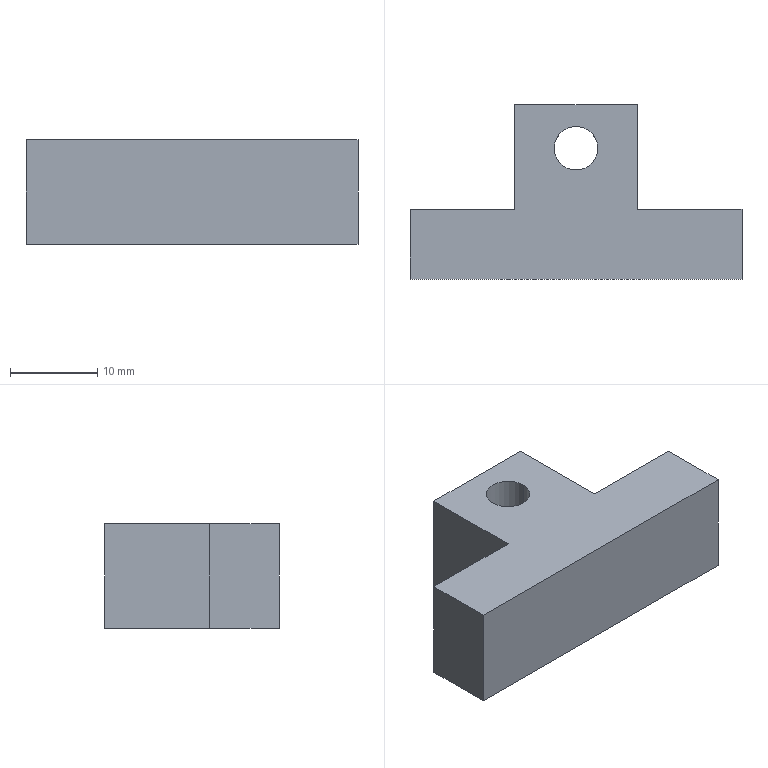Part | SolidWorks | features 3DProfileFeature 1, Extrusion 1, HoleWzd 1 | 1 solid | 12 faces | box 38 x 20 x 12 mm | volume 5428 mm3 | plane 10 | cylinder 2 | commonest cylinder face diameters 5 x2
STEP:
#1=CARTESIAN_POINT('',(-2.5,-5.,-6.));
#2=VERTEX_POINT('',#1);
#3=CARTESIAN_POINT('',(2.5,-5.,-6.));
#4=VERTEX_POINT('',#3);
#5=CARTESIAN_POINT('',(0.,-5.,-6.));
#6=DIRECTION('',(0.,0.,1.));
#7=DIRECTION('',(1.,0.,0.));
#8=AXIS2_PLACEMENT_3D('',#5,#6,#7);
#9=CIRCLE('',#8,2.5);
#10=EDGE_CURVE('',#2,#4,#9,.T.);
#11=ORIENTED_EDGE('',*,*,#10,.F.);
#12=CARTESIAN_POINT('',(-2.5,-5.,6.));
#13=VERTEX_POINT('',#12);
#14=CARTESIAN_POINT('',(-2.5,-5.,6.));
#15=DIRECTION('',(0.,0.,1.));
#16=VECTOR('',#15,1000.);
#17=LINE('',#14,#16);
#18=EDGE_CURVE('',#2,#13,#17,.T.);
#19=ORIENTED_EDGE('',*,*,#18,.T.);
#20=CARTESIAN_POINT('',(2.5,-5.,6.));
#21=VERTEX_POINT('',#20);
#22=CARTESIAN_POINT('',(0.,-5.,6.));
#23=DIRECTION('',(0.,0.,1.));
#24=DIRECTION('',(1.,0.,0.));
#25=AXIS2_PLACEMENT_3D('',#22,#23,#24);
#26=CIRCLE('',#25,2.5);
#27=EDGE_CURVE('',#13,#21,#26,.T.);
#28=ORIENTED_EDGE('',*,*,#27,.T.);
#29=CARTESIAN_POINT('',(2.5,-5.,6.));
#30=DIRECTION('',(0.,0.,1.));
#31=VECTOR('',#30,1000.);
#32=LINE('',#29,#31);
#33=EDGE_CURVE('',#4,#21,#32,.T.);
#34=ORIENTED_EDGE('',*,*,#33,.F.);
#35=EDGE_LOOP('',(#11,#19,#28,#34));
#36=FACE_OUTER_BOUND('',#35,.T.);
#37=CARTESIAN_POINT('',(0.,-5.,6.));
#38=DIRECTION('',(0.,0.,1.));
#39=DIRECTION('',(1.,0.,0.));
#40=AXIS2_PLACEMENT_3D('',#37,#38,#39);
#41=CYLINDRICAL_SURFACE('',#40,2.5);
#42=ADVANCED_FACE('',(#36),#41,.F.);
#43=CARTESIAN_POINT('',(7.,0.,-6.));
#44=VERTEX_POINT('',#43);
#45=CARTESIAN_POINT('',(-7.,0.,-6.));
#46=VERTEX_POINT('',#45);
#47=CARTESIAN_POINT('',(0.,0.,-6.));
#48=DIRECTION('',(-1.,0.,0.));
#49=VECTOR('',#48,1000.);
#50=LINE('',#47,#49);
#51=EDGE_CURVE('',#44,#46,#50,.T.);
#52=ORIENTED_EDGE('',*,*,#51,.T.);
#53=CARTESIAN_POINT('',(-7.,0.,6.));
#54=VERTEX_POINT('',#53);
#55=CARTESIAN_POINT('',(-7.,0.,6.));
#56=DIRECTION('',(0.,0.,-1.));
#57=VECTOR('',#56,1000.);
#58=LINE('',#55,#57);
#59=EDGE_CURVE('',#54,#46,#58,.T.);
#60=ORIENTED_EDGE('',*,*,#59,.F.);
#61=CARTESIAN_POINT('',(7.,0.,6.));
#62=VERTEX_POINT('',#61);
#63=CARTESIAN_POINT('',(7.,0.,6.));
#64=DIRECTION('',(-1.,0.,0.));
#65=VECTOR('',#64,1000.);
#66=LINE('',#63,#65);
#67=EDGE_CURVE('',#62,#54,#66,.T.);
#68=ORIENTED_EDGE('',*,*,#67,.F.);
#69=CARTESIAN_POINT('',(7.,0.,6.));
#70=DIRECTION('',(0.,0.,-1.));
#71=VECTOR('',#70,1000.);
#72=LINE('',#69,#71);
#73=EDGE_CURVE('',#62,#44,#72,.T.);
#74=ORIENTED_EDGE('',*,*,#73,.T.);
#75=EDGE_LOOP('',(#52,#60,#68,#74));
#76=FACE_OUTER_BOUND('',#75,.T.);
#77=CARTESIAN_POINT('',(0.,0.,6.));
#78=DIRECTION('',(0.,-1.,0.));
#79=DIRECTION('',(0.,0.,-1.));
#80=AXIS2_PLACEMENT_3D('',#77,#78,#79);
#81=PLANE('',#80);
#82=ADVANCED_FACE('',(#76),#81,.F.);
#83=CARTESIAN_POINT('',(-7.,-12.,-6.));
#84=VERTEX_POINT('',#83);
#85=CARTESIAN_POINT('',(-7.,0.,-6.));
#86=DIRECTION('',(0.,-1.,0.));
#87=VECTOR('',#86,1000.);
#88=LINE('',#85,#87);
#89=EDGE_CURVE('',#46,#84,#88,.T.);
#90=ORIENTED_EDGE('',*,*,#89,.T.);
#91=CARTESIAN_POINT('',(-7.,-12.,6.));
#92=VERTEX_POINT('',#91);
#93=CARTESIAN_POINT('',(-7.,-12.,6.));
#94=DIRECTION('',(0.,0.,-1.));
#95=VECTOR('',#94,1000.);
#96=LINE('',#93,#95);
#97=EDGE_CURVE('',#92,#84,#96,.T.);
#98=ORIENTED_EDGE('',*,*,#97,.F.);
#99=CARTESIAN_POINT('',(-7.,0.,6.));
#100=DIRECTION('',(0.,-1.,0.));
#101=VECTOR('',#100,1000.);
#102=LINE('',#99,#101);
#103=EDGE_CURVE('',#54,#92,#102,.T.);
#104=ORIENTED_EDGE('',*,*,#103,.F.);
#105=ORIENTED_EDGE('',*,*,#59,.T.);
#106=EDGE_LOOP('',(#90,#98,#104,#105));
#107=FACE_OUTER_BOUND('',#106,.T.);
#108=CARTESIAN_POINT('',(-7.,0.,6.));
#109=DIRECTION('',(1.,0.,0.));
#110=DIRECTION('',(0.,1.,0.));
#111=AXIS2_PLACEMENT_3D('',#108,#109,#110);
#112=PLANE('',#111);
#113=ADVANCED_FACE('',(#107),#112,.F.);
#114=CARTESIAN_POINT('',(-19.,-12.,-6.));
#115=VERTEX_POINT('',#114);
#116=CARTESIAN_POINT('',(-7.,-12.,-6.));
#117=DIRECTION('',(-1.,0.,0.));
#118=VECTOR('',#117,1000.);
#119=LINE('',#116,#118);
#120=EDGE_CURVE('',#84,#115,#119,.T.);
#121=ORIENTED_EDGE('',*,*,#120,.T.);
#122=CARTESIAN_POINT('',(-19.,-12.,6.));
#123=VERTEX_POINT('',#122);
#124=CARTESIAN_POINT('',(-19.,-12.,6.));
#125=DIRECTION('',(0.,0.,-1.));
#126=VECTOR('',#125,1000.);
#127=LINE('',#124,#126);
#128=EDGE_CURVE('',#123,#115,#127,.T.);
#129=ORIENTED_EDGE('',*,*,#128,.F.);
#130=CARTESIAN_POINT('',(-7.,-12.,6.));
#131=DIRECTION('',(-1.,0.,0.));
#132=VECTOR('',#131,1000.);
#133=LINE('',#130,#132);
#134=EDGE_CURVE('',#92,#123,#133,.T.);
#135=ORIENTED_EDGE('',*,*,#134,.F.);
#136=ORIENTED_EDGE('',*,*,#97,.T.);
#137=EDGE_LOOP('',(#121,#129,#135,#136));
#138=FACE_OUTER_BOUND('',#137,.T.);
#139=CARTESIAN_POINT('',(-7.,-12.,6.));
#140=DIRECTION('',(0.,-1.,0.));
#141=DIRECTION('',(1.,0.,0.));
#142=AXIS2_PLACEMENT_3D('',#139,#140,#141);
#143=PLANE('',#142);
#144=ADVANCED_FACE('',(#138),#143,.F.);
#145=CARTESIAN_POINT('',(-19.,-20.,-6.));
#146=VERTEX_POINT('',#145);
#147=CARTESIAN_POINT('',(-19.,-12.,-6.));
#148=DIRECTION('',(0.,-1.,0.));
#149=VECTOR('',#148,1000.);
#150=LINE('',#147,#149);
#151=EDGE_CURVE('',#115,#146,#150,.T.);
#152=ORIENTED_EDGE('',*,*,#151,.T.);
#153=CARTESIAN_POINT('',(-19.,-20.,6.));
#154=VERTEX_POINT('',#153);
#155=CARTESIAN_POINT('',(-19.,-20.,6.));
#156=DIRECTION('',(0.,0.,-1.));
#157=VECTOR('',#156,1000.);
#158=LINE('',#155,#157);
#159=EDGE_CURVE('',#154,#146,#158,.T.);
#160=ORIENTED_EDGE('',*,*,#159,.F.);
#161=CARTESIAN_POINT('',(-19.,-12.,6.));
#162=DIRECTION('',(0.,-1.,0.));
#163=VECTOR('',#162,1000.);
#164=LINE('',#161,#163);
#165=EDGE_CURVE('',#123,#154,#164,.T.);
#166=ORIENTED_EDGE('',*,*,#165,.F.);
#167=ORIENTED_EDGE('',*,*,#128,.T.);
#168=EDGE_LOOP('',(#152,#160,#166,#167));
#169=FACE_OUTER_BOUND('',#168,.T.);
#170=CARTESIAN_POINT('',(-19.,-12.,6.));
#171=DIRECTION('',(1.,0.,0.));
#172=DIRECTION('',(0.,0.,-1.));
#173=AXIS2_PLACEMENT_3D('',#170,#171,#172);
#174=PLANE('',#173);
#175=ADVANCED_FACE('',(#169),#174,.F.);
#176=CARTESIAN_POINT('',(19.,-20.,-6.));
#177=VERTEX_POINT('',#176);
#178=CARTESIAN_POINT('',(-19.,-20.,-6.));
#179=DIRECTION('',(1.,0.,0.));
#180=VECTOR('',#179,1000.);
#181=LINE('',#178,#180);
#182=EDGE_CURVE('',#146,#177,#181,.T.);
#183=ORIENTED_EDGE('',*,*,#182,.T.);
#184=CARTESIAN_POINT('',(19.,-20.,6.));
#185=VERTEX_POINT('',#184);
#186=CARTESIAN_POINT('',(19.,-20.,6.));
#187=DIRECTION('',(0.,0.,-1.));
#188=VECTOR('',#187,1000.);
#189=LINE('',#186,#188);
#190=EDGE_CURVE('',#185,#177,#189,.T.);
#191=ORIENTED_EDGE('',*,*,#190,.F.);
#192=CARTESIAN_POINT('',(-19.,-20.,6.));
#193=DIRECTION('',(1.,0.,0.));
#194=VECTOR('',#193,1000.);
#195=LINE('',#192,#194);
#196=EDGE_CURVE('',#154,#185,#195,.T.);
#197=ORIENTED_EDGE('',*,*,#196,.F.);
#198=ORIENTED_EDGE('',*,*,#159,.T.);
#199=EDGE_LOOP('',(#183,#191,#197,#198));
#200=FACE_OUTER_BOUND('',#199,.T.);
#201=CARTESIAN_POINT('',(-19.,-20.,6.));
#202=DIRECTION('',(0.,1.,0.));
#203=DIRECTION('',(0.,0.,1.));
#204=AXIS2_PLACEMENT_3D('',#201,#202,#203);
#205=PLANE('',#204);
#206=ADVANCED_FACE('',(#200),#205,.F.);
#207=CARTESIAN_POINT('',(19.,-12.,-6.));
#208=VERTEX_POINT('',#207);
#209=CARTESIAN_POINT('',(19.,-20.,-6.));
#210=DIRECTION('',(0.,1.,0.));
#211=VECTOR('',#210,1000.);
#212=LINE('',#209,#211);
#213=EDGE_CURVE('',#177,#208,#212,.T.);
#214=ORIENTED_EDGE('',*,*,#213,.T.);
#215=CARTESIAN_POINT('',(19.,-12.,6.));
#216=VERTEX_POINT('',#215);
#217=CARTESIAN_POINT('',(19.,-12.,6.));
#218=DIRECTION('',(0.,0.,-1.));
#219=VECTOR('',#218,1000.);
#220=LINE('',#217,#219);
#221=EDGE_CURVE('',#216,#208,#220,.T.);
#222=ORIENTED_EDGE('',*,*,#221,.F.);
#223=CARTESIAN_POINT('',(19.,-20.,6.));
#224=DIRECTION('',(0.,1.,0.));
#225=VECTOR('',#224,1000.);
#226=LINE('',#223,#225);
#227=EDGE_CURVE('',#185,#216,#226,.T.);
#228=ORIENTED_EDGE('',*,*,#227,.F.);
#229=ORIENTED_EDGE('',*,*,#190,.T.);
#230=EDGE_LOOP('',(#214,#222,#228,#229));
#231=FACE_OUTER_BOUND('',#230,.T.);
#232=CARTESIAN_POINT('',(19.,-20.,6.));
#233=DIRECTION('',(-1.,0.,0.));
#234=DIRECTION('',(0.,0.,1.));
#235=AXIS2_PLACEMENT_3D('',#232,#233,#234);
#236=PLANE('',#235);
#237=ADVANCED_FACE('',(#231),#236,.F.);
#238=CARTESIAN_POINT('',(7.,-12.,-6.));
#239=VERTEX_POINT('',#238);
#240=CARTESIAN_POINT('',(19.,-12.,-6.));
#241=DIRECTION('',(-1.,0.,0.));
#242=VECTOR('',#241,1000.);
#243=LINE('',#240,#242);
#244=EDGE_CURVE('',#208,#239,#243,.T.);
#245=ORIENTED_EDGE('',*,*,#244,.T.);
#246=CARTESIAN_POINT('',(7.,-12.,6.));
#247=VERTEX_POINT('',#246);
#248=CARTESIAN_POINT('',(7.,-12.,6.));
#249=DIRECTION('',(0.,0.,-1.));
#250=VECTOR('',#249,1000.);
#251=LINE('',#248,#250);
#252=EDGE_CURVE('',#247,#239,#251,.T.);
#253=ORIENTED_EDGE('',*,*,#252,.F.);
#254=CARTESIAN_POINT('',(19.,-12.,6.));
#255=DIRECTION('',(-1.,0.,0.));
#256=VECTOR('',#255,1000.);
#257=LINE('',#254,#256);
#258=EDGE_CURVE('',#216,#247,#257,.T.);
#259=ORIENTED_EDGE('',*,*,#258,.F.);
#260=ORIENTED_EDGE('',*,*,#221,.T.);
#261=EDGE_LOOP('',(#245,#253,#259,#260));
#262=FACE_OUTER_BOUND('',#261,.T.);
#263=CARTESIAN_POINT('',(19.,-12.,6.));
#264=DIRECTION('',(0.,-1.,0.));
#265=DIRECTION('',(0.,0.,-1.));
#266=AXIS2_PLACEMENT_3D('',#263,#264,#265);
#267=PLANE('',#266);
#268=ADVANCED_FACE('',(#262),#267,.F.);
#269=CARTESIAN_POINT('',(7.,-12.,-6.));
#270=DIRECTION('',(0.,1.,0.));
#271=VECTOR('',#270,1000.);
#272=LINE('',#269,#271);
#273=EDGE_CURVE('',#239,#44,#272,.T.);
#274=ORIENTED_EDGE('',*,*,#273,.T.);
#275=ORIENTED_EDGE('',*,*,#73,.F.);
#276=CARTESIAN_POINT('',(7.,-12.,6.));
#277=DIRECTION('',(0.,1.,0.));
#278=VECTOR('',#277,1000.);
#279=LINE('',#276,#278);
#280=EDGE_CURVE('',#247,#62,#279,.T.);
#281=ORIENTED_EDGE('',*,*,#280,.F.);
#282=ORIENTED_EDGE('',*,*,#252,.T.);
#283=EDGE_LOOP('',(#274,#275,#281,#282));
#284=FACE_OUTER_BOUND('',#283,.T.);
#285=CARTESIAN_POINT('',(7.,-12.,6.));
#286=DIRECTION('',(-1.,0.,0.));
#287=DIRECTION('',(0.,-1.,0.));
#288=AXIS2_PLACEMENT_3D('',#285,#286,#287);
#289=PLANE('',#288);
#290=ADVANCED_FACE('',(#284),#289,.F.);
#291=CARTESIAN_POINT('',(0.,-5.,6.));
#292=DIRECTION('',(0.,0.,1.));
#293=DIRECTION('',(1.,0.,0.));
#294=AXIS2_PLACEMENT_3D('',#291,#292,#293);
#295=CIRCLE('',#294,2.5);
#296=EDGE_CURVE('',#21,#13,#295,.T.);
#297=ORIENTED_EDGE('',*,*,#296,.F.);
#298=ORIENTED_EDGE('',*,*,#27,.F.);
#299=EDGE_LOOP('',(#297,#298));
#300=FACE_BOUND('',#299,.T.);
#301=ORIENTED_EDGE('',*,*,#67,.T.);
#302=ORIENTED_EDGE('',*,*,#103,.T.);
#303=ORIENTED_EDGE('',*,*,#134,.T.);
#304=ORIENTED_EDGE('',*,*,#165,.T.);
#305=ORIENTED_EDGE('',*,*,#196,.T.);
#306=ORIENTED_EDGE('',*,*,#227,.T.);
#307=ORIENTED_EDGE('',*,*,#258,.T.);
#308=ORIENTED_EDGE('',*,*,#280,.T.);
#309=EDGE_LOOP('',(#301,#302,#303,#304,#305,#306,#307,#308));
#310=FACE_OUTER_BOUND('',#309,.T.);
#311=CARTESIAN_POINT('',(0.,0.,6.));
#312=DIRECTION('',(0.,0.,1.));
#313=DIRECTION('',(1.,0.,0.));
#314=AXIS2_PLACEMENT_3D('',#311,#312,#313);
#315=PLANE('',#314);
#316=ADVANCED_FACE('',(#300,#310),#315,.T.);
#317=CARTESIAN_POINT('',(0.,-5.,-6.));
#318=DIRECTION('',(0.,0.,1.));
#319=DIRECTION('',(1.,0.,0.));
#320=AXIS2_PLACEMENT_3D('',#317,#318,#319);
#321=CIRCLE('',#320,2.5);
#322=EDGE_CURVE('',#4,#2,#321,.T.);
#323=ORIENTED_EDGE('',*,*,#322,.T.);
#324=ORIENTED_EDGE('',*,*,#10,.T.);
#325=EDGE_LOOP('',(#323,#324));
#326=FACE_BOUND('',#325,.T.);
#327=ORIENTED_EDGE('',*,*,#51,.F.);
#328=ORIENTED_EDGE('',*,*,#273,.F.);
#329=ORIENTED_EDGE('',*,*,#244,.F.);
#330=ORIENTED_EDGE('',*,*,#213,.F.);
#331=ORIENTED_EDGE('',*,*,#182,.F.);
#332=ORIENTED_EDGE('',*,*,#151,.F.);
#333=ORIENTED_EDGE('',*,*,#120,.F.);
#334=ORIENTED_EDGE('',*,*,#89,.F.);
#335=EDGE_LOOP('',(#327,#328,#329,#330,#331,#332,#333,#334));
#336=FACE_OUTER_BOUND('',#335,.T.);
#337=CARTESIAN_POINT('',(0.,0.,-6.));
#338=DIRECTION('',(0.,0.,1.));
#339=DIRECTION('',(1.,0.,0.));
#340=AXIS2_PLACEMENT_3D('',#337,#338,#339);
#341=PLANE('',#340);
#342=ADVANCED_FACE('',(#326,#336),#341,.F.);
#343=ORIENTED_EDGE('',*,*,#18,.F.);
#344=ORIENTED_EDGE('',*,*,#322,.F.);
#345=ORIENTED_EDGE('',*,*,#33,.T.);
#346=ORIENTED_EDGE('',*,*,#296,.T.);
#347=EDGE_LOOP('',(#343,#344,#345,#346));
#348=FACE_OUTER_BOUND('',#347,.T.);
#349=CARTESIAN_POINT('',(0.,-5.,6.));
#350=DIRECTION('',(0.,0.,1.));
#351=DIRECTION('',(1.,0.,0.));
#352=AXIS2_PLACEMENT_3D('',#349,#350,#351);
#353=CYLINDRICAL_SURFACE('',#352,2.5);
#354=ADVANCED_FACE('',(#348),#353,.F.);
#355=CLOSED_SHELL('',(#42,#82,#113,#144,#175,#206,#237,#268,#290,#316,#342,#354));
#356=MANIFOLD_SOLID_BREP('',#355);
#357=CARTESIAN_POINT('',(0.,0.,0.));
#358=DIRECTION('',(0.,0.,1.));
#359=DIRECTION('',(1.,0.,0.));
#360=AXIS2_PLACEMENT_3D('',#357,#358,#359);
#361=(LENGTH_UNIT()NAMED_UNIT(*)SI_UNIT(.MILLI.,.METRE.));
#362=UNCERTAINTY_MEASURE_WITH_UNIT(LENGTH_MEASURE(0.00001),#361,'','');
#363=(NAMED_UNIT(*)PLANE_ANGLE_UNIT()SI_UNIT($,.RADIAN.));
#364=(NAMED_UNIT(*)SI_UNIT($,.STERADIAN.)SOLID_ANGLE_UNIT());
#365=(GEOMETRIC_REPRESENTATION_CONTEXT(3)GLOBAL_UNCERTAINTY_ASSIGNED_CONTEXT((#362))GLOBAL_UNIT_ASSIGNED_CONTEXT((#361,#363,#364))REPRESENTATION_CONTEXT('',''));
#366=ADVANCED_BREP_SHAPE_REPRESENTATION('',(#356,#360),#365);